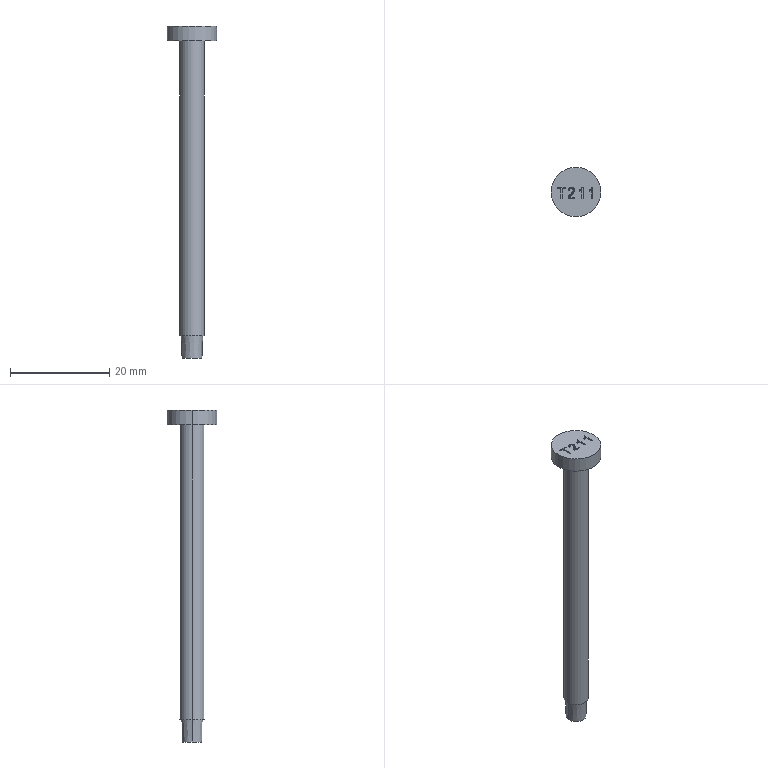Part | Creo | 1 solid | 62 faces | box 10 x 10 x 67.028 mm | volume 1465 mm3 | plane 29 | other 26 | cylinder 5 | cone 2 | commonest cylinder face diameters 5 x2 10 x2 1.927 x1